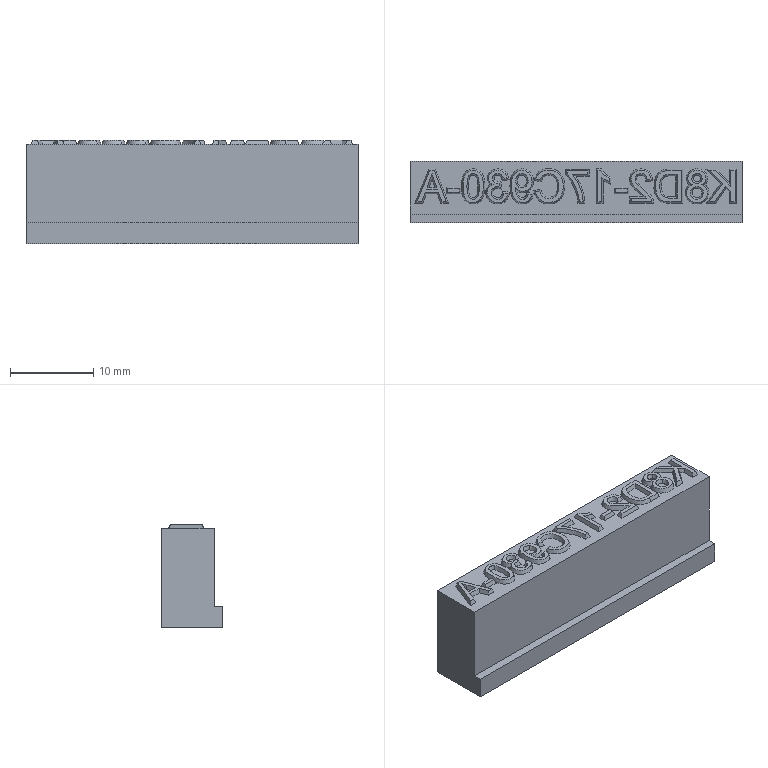Part | STEP file | lll_id502_x_t | 1 solid | 116 faces | box 40 x 7.35 x 12.5 mm | volume 3184 mm3 | plane 80 | spline 36